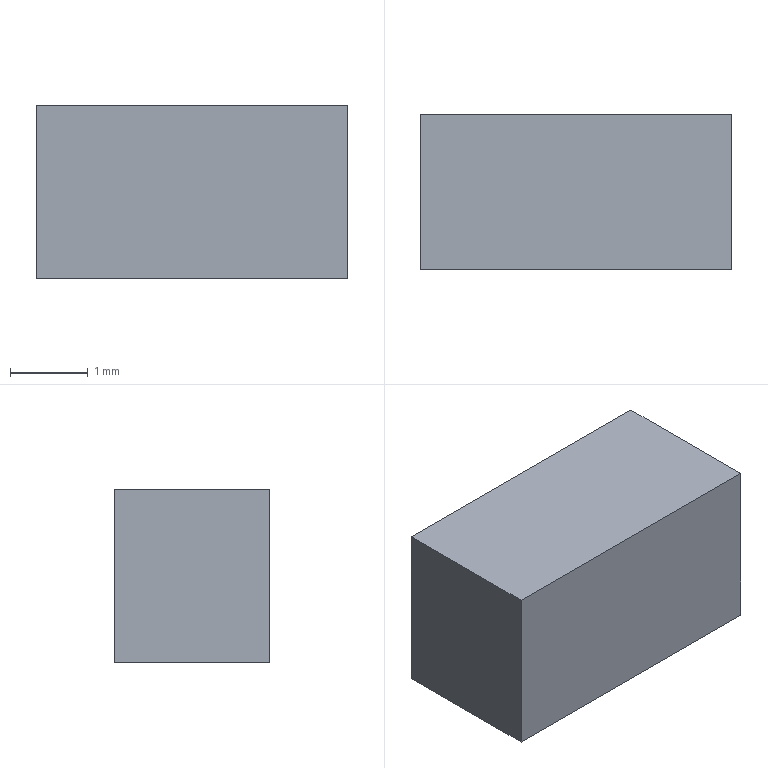Part | Creo | 1 solid | 6 faces | box 4 x 2 x 2.236 mm | volume 17.889 mm3 | plane 6
STEP:
#1=CARTESIAN_POINT('',(0.,0.,0.));
#2=DIRECTION('',(0.,0.,1.));
#3=DIRECTION('',(1.,0.,0.));
#4=AXIS2_PLACEMENT_3D('',#1,#2,#3);
#5=CARTESIAN_POINT('',(-2.,1.,0.));
#6=VERTEX_POINT('',#5);
#7=CARTESIAN_POINT('',(-2.,-1.,0.));
#8=VERTEX_POINT('',#7);
#9=CARTESIAN_POINT('',(-2.,1.,0.));
#10=DIRECTION('',(0.,-1.,0.));
#11=VECTOR('',#10,2.);
#12=LINE('',#9,#11);
#13=EDGE_CURVE('',#6,#8,#12,.T.);
#14=ORIENTED_EDGE('',*,*,#13,.T.);
#15=CARTESIAN_POINT('',(2.,-1.,0.));
#16=VERTEX_POINT('',#15);
#17=CARTESIAN_POINT('',(-2.,-1.,0.));
#18=DIRECTION('',(1.,0.,0.));
#19=VECTOR('',#18,4.);
#20=LINE('',#17,#19);
#21=EDGE_CURVE('',#8,#16,#20,.T.);
#22=ORIENTED_EDGE('',*,*,#21,.T.);
#23=CARTESIAN_POINT('',(2.,1.,0.));
#24=VERTEX_POINT('',#23);
#25=CARTESIAN_POINT('',(2.,-1.,0.));
#26=DIRECTION('',(0.,1.,0.));
#27=VECTOR('',#26,2.);
#28=LINE('',#25,#27);
#29=EDGE_CURVE('',#16,#24,#28,.T.);
#30=ORIENTED_EDGE('',*,*,#29,.T.);
#31=CARTESIAN_POINT('',(2.,1.,0.));
#32=DIRECTION('',(-1.,0.,0.));
#33=VECTOR('',#32,4.);
#34=LINE('',#31,#33);
#35=EDGE_CURVE('',#24,#6,#34,.T.);
#36=ORIENTED_EDGE('',*,*,#35,.T.);
#37=EDGE_LOOP('',(#14,#22,#30,#36));
#38=FACE_OUTER_BOUND('',#37,.F.);
#39=CARTESIAN_POINT('',(0.,0.,0.));
#40=DIRECTION('',(0.,0.,1.));
#41=DIRECTION('',(1.,0.,0.));
#42=AXIS2_PLACEMENT_3D('',#39,#40,#41);
#43=PLANE('',#42);
#44=ADVANCED_FACE('',(#38),#43,.F.);
#45=ORIENTED_EDGE('',*,*,#13,.F.);
#46=CARTESIAN_POINT('',(-2.,1.,2.236));
#47=VERTEX_POINT('',#46);
#48=CARTESIAN_POINT('',(-2.,1.,0.));
#49=DIRECTION('',(0.,0.,1.));
#50=VECTOR('',#49,2.236);
#51=LINE('',#48,#50);
#52=EDGE_CURVE('',#6,#47,#51,.T.);
#53=ORIENTED_EDGE('',*,*,#52,.T.);
#54=CARTESIAN_POINT('',(-2.,-1.,2.236));
#55=VERTEX_POINT('',#54);
#56=CARTESIAN_POINT('',(-2.,1.,2.236));
#57=DIRECTION('',(0.,-1.,0.));
#58=VECTOR('',#57,2.);
#59=LINE('',#56,#58);
#60=EDGE_CURVE('',#47,#55,#59,.T.);
#61=ORIENTED_EDGE('',*,*,#60,.T.);
#62=CARTESIAN_POINT('',(-2.,-1.,0.));
#63=DIRECTION('',(0.,0.,1.));
#64=VECTOR('',#63,2.236);
#65=LINE('',#62,#64);
#66=EDGE_CURVE('',#8,#55,#65,.T.);
#67=ORIENTED_EDGE('',*,*,#66,.F.);
#68=EDGE_LOOP('',(#45,#53,#61,#67));
#69=FACE_OUTER_BOUND('',#68,.F.);
#70=CARTESIAN_POINT('',(-2.,1.,0.));
#71=DIRECTION('',(-1.,0.,0.));
#72=DIRECTION('',(0.,-1.,0.));
#73=AXIS2_PLACEMENT_3D('',#70,#71,#72);
#74=PLANE('',#73);
#75=ADVANCED_FACE('',(#69),#74,.T.);
#76=ORIENTED_EDGE('',*,*,#35,.F.);
#77=CARTESIAN_POINT('',(2.,1.,2.236));
#78=VERTEX_POINT('',#77);
#79=CARTESIAN_POINT('',(2.,1.,0.));
#80=DIRECTION('',(0.,0.,1.));
#81=VECTOR('',#80,2.236);
#82=LINE('',#79,#81);
#83=EDGE_CURVE('',#24,#78,#82,.T.);
#84=ORIENTED_EDGE('',*,*,#83,.T.);
#85=CARTESIAN_POINT('',(2.,1.,2.236));
#86=DIRECTION('',(-1.,0.,0.));
#87=VECTOR('',#86,4.);
#88=LINE('',#85,#87);
#89=EDGE_CURVE('',#78,#47,#88,.T.);
#90=ORIENTED_EDGE('',*,*,#89,.T.);
#91=ORIENTED_EDGE('',*,*,#52,.F.);
#92=EDGE_LOOP('',(#76,#84,#90,#91));
#93=FACE_OUTER_BOUND('',#92,.F.);
#94=CARTESIAN_POINT('',(2.,1.,0.));
#95=DIRECTION('',(0.,1.,0.));
#96=DIRECTION('',(-1.,0.,0.));
#97=AXIS2_PLACEMENT_3D('',#94,#95,#96);
#98=PLANE('',#97);
#99=ADVANCED_FACE('',(#93),#98,.T.);
#100=ORIENTED_EDGE('',*,*,#29,.F.);
#101=CARTESIAN_POINT('',(2.,-1.,2.236));
#102=VERTEX_POINT('',#101);
#103=CARTESIAN_POINT('',(2.,-1.,0.));
#104=DIRECTION('',(0.,0.,1.));
#105=VECTOR('',#104,2.236);
#106=LINE('',#103,#105);
#107=EDGE_CURVE('',#16,#102,#106,.T.);
#108=ORIENTED_EDGE('',*,*,#107,.T.);
#109=CARTESIAN_POINT('',(2.,-1.,2.236));
#110=DIRECTION('',(0.,1.,0.));
#111=VECTOR('',#110,2.);
#112=LINE('',#109,#111);
#113=EDGE_CURVE('',#102,#78,#112,.T.);
#114=ORIENTED_EDGE('',*,*,#113,.T.);
#115=ORIENTED_EDGE('',*,*,#83,.F.);
#116=EDGE_LOOP('',(#100,#108,#114,#115));
#117=FACE_OUTER_BOUND('',#116,.F.);
#118=CARTESIAN_POINT('',(2.,-1.,0.));
#119=DIRECTION('',(1.,0.,0.));
#120=DIRECTION('',(0.,1.,0.));
#121=AXIS2_PLACEMENT_3D('',#118,#119,#120);
#122=PLANE('',#121);
#123=ADVANCED_FACE('',(#117),#122,.T.);
#124=ORIENTED_EDGE('',*,*,#21,.F.);
#125=ORIENTED_EDGE('',*,*,#66,.T.);
#126=CARTESIAN_POINT('',(-2.,-1.,2.236));
#127=DIRECTION('',(1.,0.,0.));
#128=VECTOR('',#127,4.);
#129=LINE('',#126,#128);
#130=EDGE_CURVE('',#55,#102,#129,.T.);
#131=ORIENTED_EDGE('',*,*,#130,.T.);
#132=ORIENTED_EDGE('',*,*,#107,.F.);
#133=EDGE_LOOP('',(#124,#125,#131,#132));
#134=FACE_OUTER_BOUND('',#133,.F.);
#135=CARTESIAN_POINT('',(-2.,-1.,0.));
#136=DIRECTION('',(0.,-1.,0.));
#137=DIRECTION('',(1.,0.,0.));
#138=AXIS2_PLACEMENT_3D('',#135,#136,#137);
#139=PLANE('',#138);
#140=ADVANCED_FACE('',(#134),#139,.T.);
#141=ORIENTED_EDGE('',*,*,#60,.F.);
#142=ORIENTED_EDGE('',*,*,#89,.F.);
#143=ORIENTED_EDGE('',*,*,#113,.F.);
#144=ORIENTED_EDGE('',*,*,#130,.F.);
#145=EDGE_LOOP('',(#141,#142,#143,#144));
#146=FACE_OUTER_BOUND('',#145,.F.);
#147=CARTESIAN_POINT('',(0.,0.,2.236));
#148=DIRECTION('',(0.,0.,1.));
#149=DIRECTION('',(1.,0.,0.));
#150=AXIS2_PLACEMENT_3D('',#147,#148,#149);
#151=PLANE('',#150);
#152=ADVANCED_FACE('',(#146),#151,.T.);
#153=CLOSED_SHELL('',(#44,#75,#99,#123,#140,#152));
#154=MANIFOLD_SOLID_BREP('',#153);
#155=(LENGTH_UNIT()NAMED_UNIT(*)SI_UNIT(.MILLI.,.METRE.));
#156=UNCERTAINTY_MEASURE_WITH_UNIT(LENGTH_MEASURE(0.0005),#155,'','');
#157=(NAMED_UNIT(*)PLANE_ANGLE_UNIT()SI_UNIT($,.RADIAN.));
#158=PLANE_ANGLE_MEASURE_WITH_UNIT(PLANE_ANGLE_MEASURE(0.01745),#157);
#159=(CONVERSION_BASED_UNIT('DEGREE',#158)NAMED_UNIT(*)PLANE_ANGLE_UNIT());
#160=(NAMED_UNIT(*)SI_UNIT($,.STERADIAN.)SOLID_ANGLE_UNIT());
#161=(GEOMETRIC_REPRESENTATION_CONTEXT(3)GLOBAL_UNCERTAINTY_ASSIGNED_CONTEXT((#156))GLOBAL_UNIT_ASSIGNED_CONTEXT((#155,#159,#160))REPRESENTATION_CONTEXT('',''));
#162=ADVANCED_BREP_SHAPE_REPRESENTATION('',(#4,#154),#161);